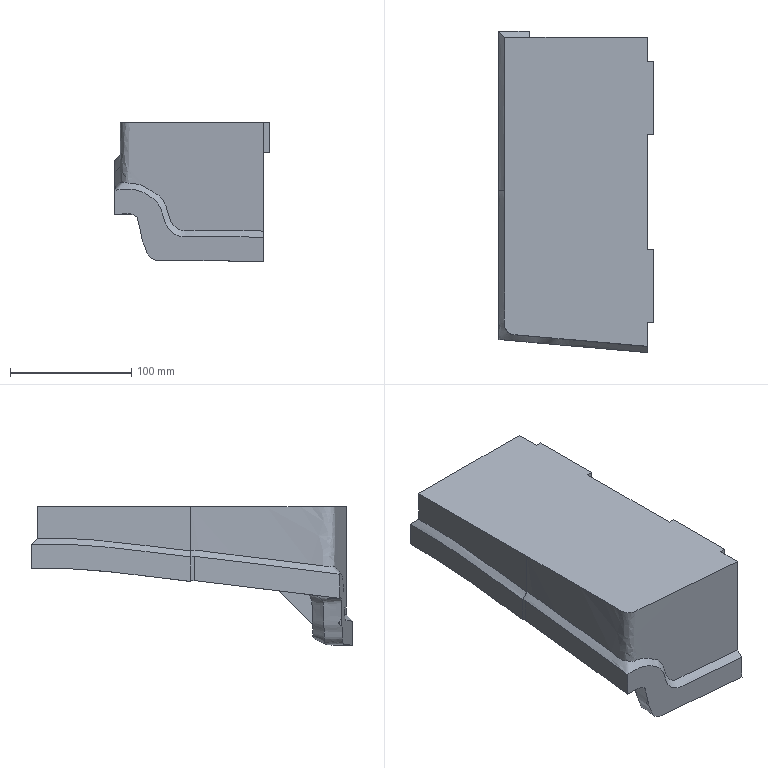Part | NX | features solid 2 | 1 solid | 46 faces | box 127.823 x 265.336 x 114.477 mm | volume 1224442 mm3 | plane 26 | spline 15 | cylinder 5 | commonest cylinder face diameters 30 x5